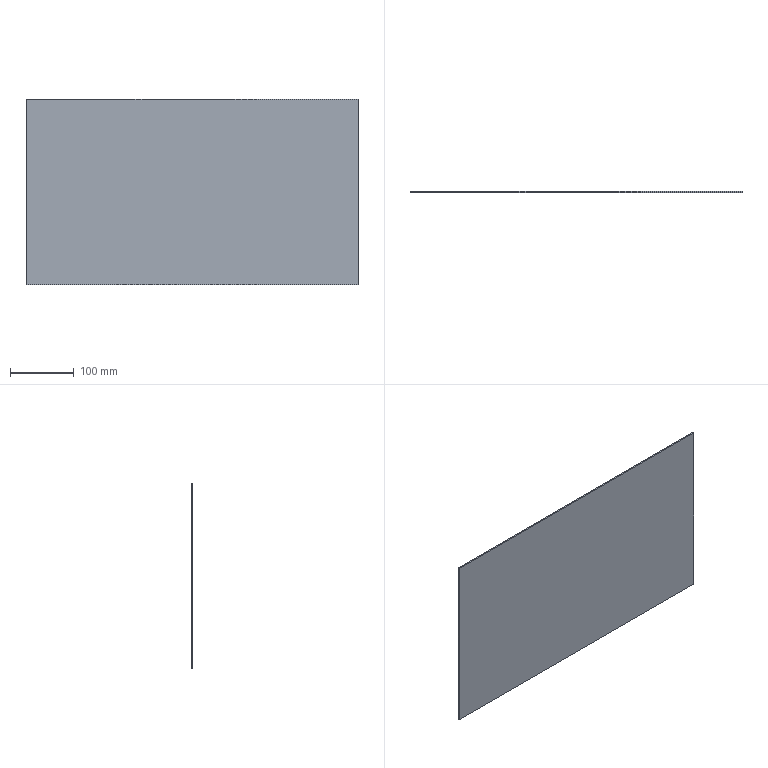Part | STEP file | Sealing plate 4 | 1 solid | 6 faces | box 520 x 2 x 290 mm | volume 301600 mm3 | plane 6
STEP:
#1=CARTESIAN_POINT('',(0.,0.,0.));
#2=DIRECTION('',(0.,0.,1.));
#3=DIRECTION('',(1.,0.,0.));
#4=AXIS2_PLACEMENT_3D('',#1,#2,#3);
#5=CARTESIAN_POINT('',(0.,0.,0.));
#6=VERTEX_POINT('',#5);
#7=CARTESIAN_POINT('',(0.,0.,290.));
#8=VERTEX_POINT('',#7);
#9=CARTESIAN_POINT('',(0.,0.,0.));
#10=DIRECTION('',(0.,0.,1.));
#11=VECTOR('',#10,1.);
#12=LINE('',#9,#11);
#13=CARTESIAN_POINT('',(0.,2.,0.));
#14=DIRECTION('',(1.,0.,0.));
#15=DIRECTION('',(0.,0.,-1.));
#16=AXIS2_PLACEMENT_3D('',#13,#14,#15);
#17=PLANE('',#16);
#18=CARTESIAN_POINT('',(0.,-2.));
#19=DIRECTION('',(-1.,0.));
#20=VECTOR('',#19,1.);
#21=LINE('',#18,#20);
#22=(GEOMETRIC_REPRESENTATION_CONTEXT(2)PARAMETRIC_REPRESENTATION_CONTEXT()REPRESENTATION_CONTEXT('',''));
#23=DEFINITIONAL_REPRESENTATION('',(#21),#22);
#24=PCURVE('',#17,#23);
#25=CARTESIAN_POINT('',(0.,0.,0.));
#26=DIRECTION('',(0.,1.,0.));
#27=DIRECTION('',(0.,0.,1.));
#28=AXIS2_PLACEMENT_3D('',#25,#26,#27);
#29=PLANE('',#28);
#30=CARTESIAN_POINT('',(0.,0.));
#31=DIRECTION('',(1.,0.));
#32=VECTOR('',#31,1.);
#33=LINE('',#30,#32);
#34=(GEOMETRIC_REPRESENTATION_CONTEXT(2)PARAMETRIC_REPRESENTATION_CONTEXT()REPRESENTATION_CONTEXT('',''));
#35=DEFINITIONAL_REPRESENTATION('',(#33),#34);
#36=PCURVE('',#29,#35);
#37=SURFACE_CURVE('',#12,(#24,#36),.PCURVE_S1.);
#38=EDGE_CURVE('',#6,#8,#37,.T.);
#39=ORIENTED_EDGE('',*,*,#38,.T.);
#40=CARTESIAN_POINT('',(0.,2.,290.));
#41=VERTEX_POINT('',#40);
#42=CARTESIAN_POINT('',(0.,2.,290.));
#43=DIRECTION('',(0.,-1.,0.));
#44=VECTOR('',#43,1.);
#45=LINE('',#42,#44);
#46=CARTESIAN_POINT('',(-290.,0.));
#47=DIRECTION('',(0.,-1.));
#48=VECTOR('',#47,1.);
#49=LINE('',#46,#48);
#50=(GEOMETRIC_REPRESENTATION_CONTEXT(2)PARAMETRIC_REPRESENTATION_CONTEXT()REPRESENTATION_CONTEXT('',''));
#51=DEFINITIONAL_REPRESENTATION('',(#49),#50);
#52=PCURVE('',#17,#51);
#53=CARTESIAN_POINT('',(0.,2.,290.));
#54=DIRECTION('',(0.,0.,-1.));
#55=DIRECTION('',(-1.,0.,0.));
#56=AXIS2_PLACEMENT_3D('',#53,#54,#55);
#57=PLANE('',#56);
#58=CARTESIAN_POINT('',(0.,0.));
#59=DIRECTION('',(0.,-1.));
#60=VECTOR('',#59,1.);
#61=LINE('',#58,#60);
#62=(GEOMETRIC_REPRESENTATION_CONTEXT(2)PARAMETRIC_REPRESENTATION_CONTEXT()REPRESENTATION_CONTEXT('',''));
#63=DEFINITIONAL_REPRESENTATION('',(#61),#62);
#64=PCURVE('',#57,#63);
#65=SURFACE_CURVE('',#45,(#52,#64),.PCURVE_S1.);
#66=EDGE_CURVE('',#41,#8,#65,.T.);
#67=ORIENTED_EDGE('',*,*,#66,.F.);
#68=CARTESIAN_POINT('',(0.,2.,0.));
#69=VERTEX_POINT('',#68);
#70=CARTESIAN_POINT('',(0.,2.,0.));
#71=DIRECTION('',(0.,0.,1.));
#72=VECTOR('',#71,1.);
#73=LINE('',#70,#72);
#74=CARTESIAN_POINT('',(0.,0.));
#75=DIRECTION('',(-1.,0.));
#76=VECTOR('',#75,1.);
#77=LINE('',#74,#76);
#78=(GEOMETRIC_REPRESENTATION_CONTEXT(2)PARAMETRIC_REPRESENTATION_CONTEXT()REPRESENTATION_CONTEXT('',''));
#79=DEFINITIONAL_REPRESENTATION('',(#77),#78);
#80=PCURVE('',#17,#79);
#81=CARTESIAN_POINT('',(0.,2.,0.));
#82=DIRECTION('',(0.,1.,0.));
#83=DIRECTION('',(0.,0.,1.));
#84=AXIS2_PLACEMENT_3D('',#81,#82,#83);
#85=PLANE('',#84);
#86=CARTESIAN_POINT('',(0.,0.));
#87=DIRECTION('',(1.,0.));
#88=VECTOR('',#87,1.);
#89=LINE('',#86,#88);
#90=(GEOMETRIC_REPRESENTATION_CONTEXT(2)PARAMETRIC_REPRESENTATION_CONTEXT()REPRESENTATION_CONTEXT('',''));
#91=DEFINITIONAL_REPRESENTATION('',(#89),#90);
#92=PCURVE('',#85,#91);
#93=SURFACE_CURVE('',#73,(#80,#92),.PCURVE_S1.);
#94=EDGE_CURVE('',#69,#41,#93,.T.);
#95=ORIENTED_EDGE('',*,*,#94,.F.);
#96=CARTESIAN_POINT('',(0.,2.,0.));
#97=DIRECTION('',(0.,-1.,0.));
#98=VECTOR('',#97,1.);
#99=LINE('',#96,#98);
#100=CARTESIAN_POINT('',(0.,0.));
#101=DIRECTION('',(0.,-1.));
#102=VECTOR('',#101,1.);
#103=LINE('',#100,#102);
#104=(GEOMETRIC_REPRESENTATION_CONTEXT(2)PARAMETRIC_REPRESENTATION_CONTEXT()REPRESENTATION_CONTEXT('',''));
#105=DEFINITIONAL_REPRESENTATION('',(#103),#104);
#106=PCURVE('',#17,#105);
#107=CARTESIAN_POINT('',(0.,2.,0.));
#108=DIRECTION('',(0.,0.,1.));
#109=DIRECTION('',(1.,0.,0.));
#110=AXIS2_PLACEMENT_3D('',#107,#108,#109);
#111=PLANE('',#110);
#112=CARTESIAN_POINT('',(0.,0.));
#113=DIRECTION('',(0.,-1.));
#114=VECTOR('',#113,1.);
#115=LINE('',#112,#114);
#116=(GEOMETRIC_REPRESENTATION_CONTEXT(2)PARAMETRIC_REPRESENTATION_CONTEXT()REPRESENTATION_CONTEXT('',''));
#117=DEFINITIONAL_REPRESENTATION('',(#115),#116);
#118=PCURVE('',#111,#117);
#119=SURFACE_CURVE('',#99,(#106,#118),.PCURVE_S1.);
#120=EDGE_CURVE('',#69,#6,#119,.T.);
#121=ORIENTED_EDGE('',*,*,#120,.T.);
#122=EDGE_LOOP('',(#39,#67,#95,#121));
#123=FACE_BOUND('',#122,.T.);
#124=ADVANCED_FACE('',(#123),#17,.F.);
#125=CARTESIAN_POINT('',(520.,0.,290.));
#126=VERTEX_POINT('',#125);
#127=CARTESIAN_POINT('',(0.,0.,290.));
#128=DIRECTION('',(1.,0.,0.));
#129=VECTOR('',#128,1.);
#130=LINE('',#127,#129);
#131=CARTESIAN_POINT('',(0.,-2.));
#132=DIRECTION('',(-1.,0.));
#133=VECTOR('',#132,1.);
#134=LINE('',#131,#133);
#135=(GEOMETRIC_REPRESENTATION_CONTEXT(2)PARAMETRIC_REPRESENTATION_CONTEXT()REPRESENTATION_CONTEXT('',''));
#136=DEFINITIONAL_REPRESENTATION('',(#134),#135);
#137=PCURVE('',#57,#136);
#138=CARTESIAN_POINT('',(290.,0.));
#139=DIRECTION('',(0.,1.));
#140=VECTOR('',#139,1.);
#141=LINE('',#138,#140);
#142=(GEOMETRIC_REPRESENTATION_CONTEXT(2)PARAMETRIC_REPRESENTATION_CONTEXT()REPRESENTATION_CONTEXT('',''));
#143=DEFINITIONAL_REPRESENTATION('',(#141),#142);
#144=PCURVE('',#29,#143);
#145=SURFACE_CURVE('',#130,(#137,#144),.PCURVE_S1.);
#146=EDGE_CURVE('',#8,#126,#145,.T.);
#147=ORIENTED_EDGE('',*,*,#146,.T.);
#148=CARTESIAN_POINT('',(520.,2.,290.));
#149=VERTEX_POINT('',#148);
#150=CARTESIAN_POINT('',(520.,2.,290.));
#151=DIRECTION('',(0.,-1.,0.));
#152=VECTOR('',#151,1.);
#153=LINE('',#150,#152);
#154=CARTESIAN_POINT('',(-520.,0.));
#155=DIRECTION('',(0.,-1.));
#156=VECTOR('',#155,1.);
#157=LINE('',#154,#156);
#158=(GEOMETRIC_REPRESENTATION_CONTEXT(2)PARAMETRIC_REPRESENTATION_CONTEXT()REPRESENTATION_CONTEXT('',''));
#159=DEFINITIONAL_REPRESENTATION('',(#157),#158);
#160=PCURVE('',#57,#159);
#161=CARTESIAN_POINT('',(520.,2.,0.));
#162=DIRECTION('',(-1.,0.,0.));
#163=DIRECTION('',(0.,0.,1.));
#164=AXIS2_PLACEMENT_3D('',#161,#162,#163);
#165=PLANE('',#164);
#166=CARTESIAN_POINT('',(290.,0.));
#167=DIRECTION('',(0.,-1.));
#168=VECTOR('',#167,1.);
#169=LINE('',#166,#168);
#170=(GEOMETRIC_REPRESENTATION_CONTEXT(2)PARAMETRIC_REPRESENTATION_CONTEXT()REPRESENTATION_CONTEXT('',''));
#171=DEFINITIONAL_REPRESENTATION('',(#169),#170);
#172=PCURVE('',#165,#171);
#173=SURFACE_CURVE('',#153,(#160,#172),.PCURVE_S1.);
#174=EDGE_CURVE('',#149,#126,#173,.T.);
#175=ORIENTED_EDGE('',*,*,#174,.F.);
#176=CARTESIAN_POINT('',(0.,2.,290.));
#177=DIRECTION('',(1.,0.,0.));
#178=VECTOR('',#177,1.);
#179=LINE('',#176,#178);
#180=CARTESIAN_POINT('',(0.,0.));
#181=DIRECTION('',(-1.,0.));
#182=VECTOR('',#181,1.);
#183=LINE('',#180,#182);
#184=(GEOMETRIC_REPRESENTATION_CONTEXT(2)PARAMETRIC_REPRESENTATION_CONTEXT()REPRESENTATION_CONTEXT('',''));
#185=DEFINITIONAL_REPRESENTATION('',(#183),#184);
#186=PCURVE('',#57,#185);
#187=CARTESIAN_POINT('',(290.,0.));
#188=DIRECTION('',(0.,1.));
#189=VECTOR('',#188,1.);
#190=LINE('',#187,#189);
#191=(GEOMETRIC_REPRESENTATION_CONTEXT(2)PARAMETRIC_REPRESENTATION_CONTEXT()REPRESENTATION_CONTEXT('',''));
#192=DEFINITIONAL_REPRESENTATION('',(#190),#191);
#193=PCURVE('',#85,#192);
#194=SURFACE_CURVE('',#179,(#186,#193),.PCURVE_S1.);
#195=EDGE_CURVE('',#41,#149,#194,.T.);
#196=ORIENTED_EDGE('',*,*,#195,.F.);
#197=ORIENTED_EDGE('',*,*,#66,.T.);
#198=EDGE_LOOP('',(#147,#175,#196,#197));
#199=FACE_BOUND('',#198,.T.);
#200=ADVANCED_FACE('',(#199),#57,.F.);
#201=CARTESIAN_POINT('',(520.,0.,0.));
#202=VERTEX_POINT('',#201);
#203=CARTESIAN_POINT('',(520.,0.,0.));
#204=DIRECTION('',(0.,0.,-1.));
#205=VECTOR('',#204,1.);
#206=LINE('',#203,#205);
#207=CARTESIAN_POINT('',(0.,-2.));
#208=DIRECTION('',(-1.,0.));
#209=VECTOR('',#208,1.);
#210=LINE('',#207,#209);
#211=(GEOMETRIC_REPRESENTATION_CONTEXT(2)PARAMETRIC_REPRESENTATION_CONTEXT()REPRESENTATION_CONTEXT('',''));
#212=DEFINITIONAL_REPRESENTATION('',(#210),#211);
#213=PCURVE('',#165,#212);
#214=CARTESIAN_POINT('',(0.,520.));
#215=DIRECTION('',(-1.,0.));
#216=VECTOR('',#215,1.);
#217=LINE('',#214,#216);
#218=(GEOMETRIC_REPRESENTATION_CONTEXT(2)PARAMETRIC_REPRESENTATION_CONTEXT()REPRESENTATION_CONTEXT('',''));
#219=DEFINITIONAL_REPRESENTATION('',(#217),#218);
#220=PCURVE('',#29,#219);
#221=SURFACE_CURVE('',#206,(#213,#220),.PCURVE_S1.);
#222=EDGE_CURVE('',#126,#202,#221,.T.);
#223=ORIENTED_EDGE('',*,*,#222,.T.);
#224=CARTESIAN_POINT('',(520.,2.,0.));
#225=VERTEX_POINT('',#224);
#226=CARTESIAN_POINT('',(520.,2.,0.));
#227=DIRECTION('',(0.,-1.,0.));
#228=VECTOR('',#227,1.);
#229=LINE('',#226,#228);
#230=CARTESIAN_POINT('',(0.,0.));
#231=DIRECTION('',(0.,-1.));
#232=VECTOR('',#231,1.);
#233=LINE('',#230,#232);
#234=(GEOMETRIC_REPRESENTATION_CONTEXT(2)PARAMETRIC_REPRESENTATION_CONTEXT()REPRESENTATION_CONTEXT('',''));
#235=DEFINITIONAL_REPRESENTATION('',(#233),#234);
#236=PCURVE('',#165,#235);
#237=CARTESIAN_POINT('',(520.,0.));
#238=DIRECTION('',(0.,-1.));
#239=VECTOR('',#238,1.);
#240=LINE('',#237,#239);
#241=(GEOMETRIC_REPRESENTATION_CONTEXT(2)PARAMETRIC_REPRESENTATION_CONTEXT()REPRESENTATION_CONTEXT('',''));
#242=DEFINITIONAL_REPRESENTATION('',(#240),#241);
#243=PCURVE('',#111,#242);
#244=SURFACE_CURVE('',#229,(#236,#243),.PCURVE_S1.);
#245=EDGE_CURVE('',#225,#202,#244,.T.);
#246=ORIENTED_EDGE('',*,*,#245,.F.);
#247=CARTESIAN_POINT('',(520.,2.,0.));
#248=DIRECTION('',(0.,0.,-1.));
#249=VECTOR('',#248,1.);
#250=LINE('',#247,#249);
#251=CARTESIAN_POINT('',(0.,0.));
#252=DIRECTION('',(-1.,0.));
#253=VECTOR('',#252,1.);
#254=LINE('',#251,#253);
#255=(GEOMETRIC_REPRESENTATION_CONTEXT(2)PARAMETRIC_REPRESENTATION_CONTEXT()REPRESENTATION_CONTEXT('',''));
#256=DEFINITIONAL_REPRESENTATION('',(#254),#255);
#257=PCURVE('',#165,#256);
#258=CARTESIAN_POINT('',(0.,520.));
#259=DIRECTION('',(-1.,0.));
#260=VECTOR('',#259,1.);
#261=LINE('',#258,#260);
#262=(GEOMETRIC_REPRESENTATION_CONTEXT(2)PARAMETRIC_REPRESENTATION_CONTEXT()REPRESENTATION_CONTEXT('',''));
#263=DEFINITIONAL_REPRESENTATION('',(#261),#262);
#264=PCURVE('',#85,#263);
#265=SURFACE_CURVE('',#250,(#257,#264),.PCURVE_S1.);
#266=EDGE_CURVE('',#149,#225,#265,.T.);
#267=ORIENTED_EDGE('',*,*,#266,.F.);
#268=ORIENTED_EDGE('',*,*,#174,.T.);
#269=EDGE_LOOP('',(#223,#246,#267,#268));
#270=FACE_BOUND('',#269,.T.);
#271=ADVANCED_FACE('',(#270),#165,.F.);
#272=CARTESIAN_POINT('',(0.,0.,0.));
#273=DIRECTION('',(-1.,0.,0.));
#274=VECTOR('',#273,1.);
#275=LINE('',#272,#274);
#276=CARTESIAN_POINT('',(0.,-2.));
#277=DIRECTION('',(-1.,0.));
#278=VECTOR('',#277,1.);
#279=LINE('',#276,#278);
#280=(GEOMETRIC_REPRESENTATION_CONTEXT(2)PARAMETRIC_REPRESENTATION_CONTEXT()REPRESENTATION_CONTEXT('',''));
#281=DEFINITIONAL_REPRESENTATION('',(#279),#280);
#282=PCURVE('',#111,#281);
#283=CARTESIAN_POINT('',(0.,0.));
#284=DIRECTION('',(0.,-1.));
#285=VECTOR('',#284,1.);
#286=LINE('',#283,#285);
#287=(GEOMETRIC_REPRESENTATION_CONTEXT(2)PARAMETRIC_REPRESENTATION_CONTEXT()REPRESENTATION_CONTEXT('',''));
#288=DEFINITIONAL_REPRESENTATION('',(#286),#287);
#289=PCURVE('',#29,#288);
#290=SURFACE_CURVE('',#275,(#282,#289),.PCURVE_S1.);
#291=EDGE_CURVE('',#202,#6,#290,.T.);
#292=ORIENTED_EDGE('',*,*,#291,.T.);
#293=ORIENTED_EDGE('',*,*,#120,.F.);
#294=CARTESIAN_POINT('',(0.,2.,0.));
#295=DIRECTION('',(-1.,0.,0.));
#296=VECTOR('',#295,1.);
#297=LINE('',#294,#296);
#298=CARTESIAN_POINT('',(0.,0.));
#299=DIRECTION('',(-1.,0.));
#300=VECTOR('',#299,1.);
#301=LINE('',#298,#300);
#302=(GEOMETRIC_REPRESENTATION_CONTEXT(2)PARAMETRIC_REPRESENTATION_CONTEXT()REPRESENTATION_CONTEXT('',''));
#303=DEFINITIONAL_REPRESENTATION('',(#301),#302);
#304=PCURVE('',#111,#303);
#305=CARTESIAN_POINT('',(0.,0.));
#306=DIRECTION('',(0.,-1.));
#307=VECTOR('',#306,1.);
#308=LINE('',#305,#307);
#309=(GEOMETRIC_REPRESENTATION_CONTEXT(2)PARAMETRIC_REPRESENTATION_CONTEXT()REPRESENTATION_CONTEXT('',''));
#310=DEFINITIONAL_REPRESENTATION('',(#308),#309);
#311=PCURVE('',#85,#310);
#312=SURFACE_CURVE('',#297,(#304,#311),.PCURVE_S1.);
#313=EDGE_CURVE('',#225,#69,#312,.T.);
#314=ORIENTED_EDGE('',*,*,#313,.F.);
#315=ORIENTED_EDGE('',*,*,#245,.T.);
#316=EDGE_LOOP('',(#292,#293,#314,#315));
#317=FACE_BOUND('',#316,.T.);
#318=ADVANCED_FACE('',(#317),#111,.F.);
#319=ORIENTED_EDGE('',*,*,#94,.T.);
#320=ORIENTED_EDGE('',*,*,#195,.T.);
#321=ORIENTED_EDGE('',*,*,#266,.T.);
#322=ORIENTED_EDGE('',*,*,#313,.T.);
#323=EDGE_LOOP('',(#319,#320,#321,#322));
#324=FACE_BOUND('',#323,.T.);
#325=ADVANCED_FACE('',(#324),#85,.T.);
#326=ORIENTED_EDGE('',*,*,#38,.F.);
#327=ORIENTED_EDGE('',*,*,#291,.F.);
#328=ORIENTED_EDGE('',*,*,#222,.F.);
#329=ORIENTED_EDGE('',*,*,#146,.F.);
#330=EDGE_LOOP('',(#326,#327,#328,#329));
#331=FACE_BOUND('',#330,.T.);
#332=ADVANCED_FACE('',(#331),#29,.F.);
#333=CLOSED_SHELL('',(#124,#200,#271,#318,#325,#332));
#334=MANIFOLD_SOLID_BREP('',#333);
#335=(LENGTH_UNIT()NAMED_UNIT(*)SI_UNIT(.MILLI.,.METRE.));
#336=UNCERTAINTY_MEASURE_WITH_UNIT(LENGTH_MEASURE(0.0000001),#335,'','');
#337=(NAMED_UNIT(*)PLANE_ANGLE_UNIT()SI_UNIT($,.RADIAN.));
#338=(NAMED_UNIT(*)SI_UNIT($,.STERADIAN.)SOLID_ANGLE_UNIT());
#339=(GEOMETRIC_REPRESENTATION_CONTEXT(3)GLOBAL_UNCERTAINTY_ASSIGNED_CONTEXT((#336))GLOBAL_UNIT_ASSIGNED_CONTEXT((#335,#337,#338))REPRESENTATION_CONTEXT('',''));
#340=ADVANCED_BREP_SHAPE_REPRESENTATION('',(#4,#334),#339);